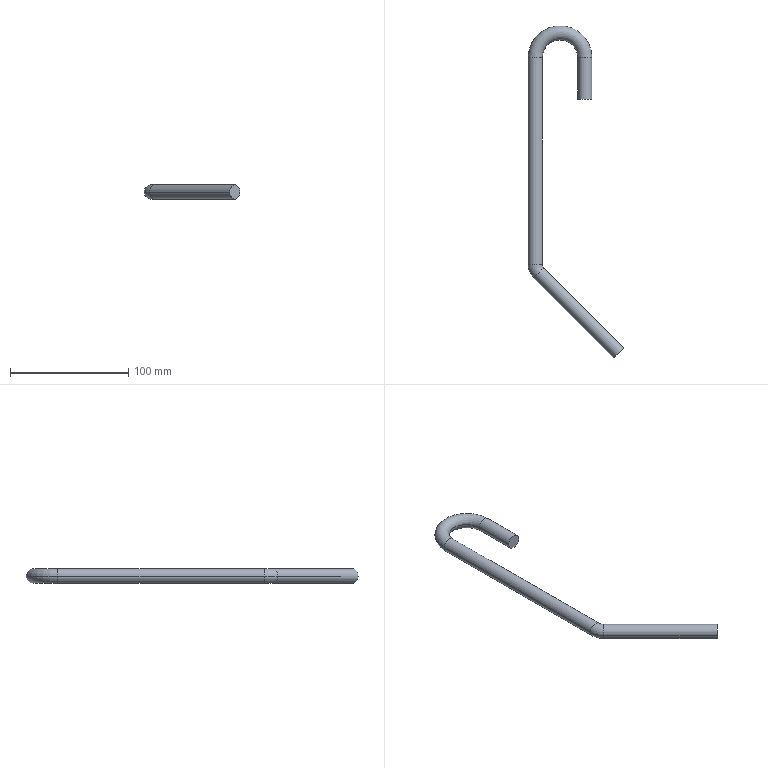Part | SolidWorks | features Sweep 1 | 1 solid | 12 faces | box 80.953 x 280.953 x 12 mm | volume 42925 mm3 | cylinder 6 | torus 4 | plane 2 | commonest cylinder face diameters 12 x6
STEP:
#1=CARTESIAN_POINT('',(-76.711,249.711,0.));
#2=VERTEX_POINT('',#1);
#3=CARTESIAN_POINT('',(-64.711,249.711,0.));
#4=VERTEX_POINT('',#3);
#5=CARTESIAN_POINT('',(-70.711,249.711,0.));
#6=DIRECTION('',(0.,-1.,0.));
#7=DIRECTION('',(0.,0.,1.));
#8=AXIS2_PLACEMENT_3D('',#5,#6,#7);
#9=CIRCLE('',#8,6.);
#10=EDGE_CURVE('',#2,#4,#9,.T.);
#11=ORIENTED_EDGE('',*,*,#10,.F.);
#12=CARTESIAN_POINT('',(-22.711,249.711,0.));
#13=VERTEX_POINT('',#12);
#14=CARTESIAN_POINT('',(-49.711,249.711,0.));
#15=DIRECTION('',(0.,0.,-1.));
#16=DIRECTION('',(-1.,0.,0.));
#17=AXIS2_PLACEMENT_3D('',#14,#15,#16);
#18=CIRCLE('',#17,27.);
#19=EDGE_CURVE('',#2,#13,#18,.T.);
#20=ORIENTED_EDGE('',*,*,#19,.T.);
#21=CARTESIAN_POINT('',(-34.711,249.711,0.));
#22=VERTEX_POINT('',#21);
#23=CARTESIAN_POINT('',(-28.711,249.711,0.));
#24=DIRECTION('',(0.,1.,0.));
#25=DIRECTION('',(0.,0.,1.));
#26=AXIS2_PLACEMENT_3D('',#23,#24,#25);
#27=CIRCLE('',#26,6.);
#28=EDGE_CURVE('',#13,#22,#27,.T.);
#29=ORIENTED_EDGE('',*,*,#28,.T.);
#30=CARTESIAN_POINT('',(-49.711,249.711,0.));
#31=DIRECTION('',(0.,0.,-1.));
#32=DIRECTION('',(-1.,0.,0.));
#33=AXIS2_PLACEMENT_3D('',#30,#31,#32);
#34=CIRCLE('',#33,15.);
#35=EDGE_CURVE('',#4,#22,#34,.T.);
#36=ORIENTED_EDGE('',*,*,#35,.F.);
#37=EDGE_LOOP('',(#11,#20,#29,#36));
#38=FACE_OUTER_BOUND('',#37,.T.);
#39=CARTESIAN_POINT('',(-49.711,249.711,0.));
#40=DIRECTION('',(0.,0.,-1.));
#41=DIRECTION('',(-1.,0.,0.));
#42=AXIS2_PLACEMENT_3D('',#39,#40,#41);
#43=TOROIDAL_SURFACE('',#42,21.,6.);
#44=ADVANCED_FACE('',(#38),#43,.T.);
#45=CARTESIAN_POINT('',(-72.024,63.539,0.));
#46=VERTEX_POINT('',#45);
#47=CARTESIAN_POINT('',(-63.539,72.024,0.));
#48=VERTEX_POINT('',#47);
#49=CARTESIAN_POINT('',(-67.782,67.782,0.));
#50=DIRECTION('',(0.7071,-0.7071,0.));
#51=DIRECTION('',(0.,0.,1.));
#52=AXIS2_PLACEMENT_3D('',#49,#50,#51);
#53=CIRCLE('',#52,6.);
#54=EDGE_CURVE('',#46,#48,#53,.T.);
#55=ORIENTED_EDGE('',*,*,#54,.F.);
#56=CARTESIAN_POINT('',(-76.711,74.853,0.));
#57=VERTEX_POINT('',#56);
#58=CARTESIAN_POINT('',(-60.711,74.853,0.));
#59=DIRECTION('',(0.,0.,-1.));
#60=DIRECTION('',(-1.,0.,0.));
#61=AXIS2_PLACEMENT_3D('',#58,#59,#60);
#62=CIRCLE('',#61,16.);
#63=EDGE_CURVE('',#46,#57,#62,.T.);
#64=ORIENTED_EDGE('',*,*,#63,.T.);
#65=CARTESIAN_POINT('',(-64.711,74.853,0.));
#66=VERTEX_POINT('',#65);
#67=CARTESIAN_POINT('',(-70.711,74.853,0.));
#68=DIRECTION('',(0.,-1.,0.));
#69=DIRECTION('',(0.,0.,1.));
#70=AXIS2_PLACEMENT_3D('',#67,#68,#69);
#71=CIRCLE('',#70,6.);
#72=EDGE_CURVE('',#57,#66,#71,.T.);
#73=ORIENTED_EDGE('',*,*,#72,.T.);
#74=CARTESIAN_POINT('',(-60.711,74.853,0.));
#75=DIRECTION('',(0.,0.,-1.));
#76=DIRECTION('',(-1.,0.,0.));
#77=AXIS2_PLACEMENT_3D('',#74,#75,#76);
#78=CIRCLE('',#77,4.);
#79=EDGE_CURVE('',#48,#66,#78,.T.);
#80=ORIENTED_EDGE('',*,*,#79,.F.);
#81=EDGE_LOOP('',(#55,#64,#73,#80));
#82=FACE_OUTER_BOUND('',#81,.T.);
#83=CARTESIAN_POINT('',(-60.711,74.853,0.));
#84=DIRECTION('',(0.,0.,-1.));
#85=DIRECTION('',(-1.,0.,0.));
#86=AXIS2_PLACEMENT_3D('',#83,#84,#85);
#87=TOROIDAL_SURFACE('',#86,10.,6.);
#88=ADVANCED_FACE('',(#82),#87,.T.);
#89=CARTESIAN_POINT('',(-28.711,249.711,0.));
#90=DIRECTION('',(0.,1.,0.));
#91=DIRECTION('',(0.,0.,1.));
#92=AXIS2_PLACEMENT_3D('',#89,#90,#91);
#93=CIRCLE('',#92,6.);
#94=EDGE_CURVE('',#22,#13,#93,.T.);
#95=ORIENTED_EDGE('',*,*,#94,.F.);
#96=CARTESIAN_POINT('',(-34.711,214.711,0.));
#97=VERTEX_POINT('',#96);
#98=CARTESIAN_POINT('',(-34.711,249.711,0.));
#99=DIRECTION('',(0.,-1.,0.));
#100=VECTOR('',#99,1000.);
#101=LINE('',#98,#100);
#102=EDGE_CURVE('',#22,#97,#101,.T.);
#103=ORIENTED_EDGE('',*,*,#102,.T.);
#104=CARTESIAN_POINT('',(-22.711,214.711,0.));
#105=VERTEX_POINT('',#104);
#106=CARTESIAN_POINT('',(-28.711,214.711,0.));
#107=DIRECTION('',(0.,1.,0.));
#108=DIRECTION('',(0.,0.,1.));
#109=AXIS2_PLACEMENT_3D('',#106,#107,#108);
#110=CIRCLE('',#109,6.);
#111=EDGE_CURVE('',#97,#105,#110,.T.);
#112=ORIENTED_EDGE('',*,*,#111,.T.);
#113=CARTESIAN_POINT('',(-22.711,249.711,0.));
#114=DIRECTION('',(0.,-1.,0.));
#115=VECTOR('',#114,1000.);
#116=LINE('',#113,#115);
#117=EDGE_CURVE('',#13,#105,#116,.T.);
#118=ORIENTED_EDGE('',*,*,#117,.F.);
#119=EDGE_LOOP('',(#95,#103,#112,#118));
#120=FACE_OUTER_BOUND('',#119,.T.);
#121=CARTESIAN_POINT('',(-28.711,249.711,0.));
#122=DIRECTION('',(0.,-1.,0.));
#123=DIRECTION('',(1.,0.,0.));
#124=AXIS2_PLACEMENT_3D('',#121,#122,#123);
#125=CYLINDRICAL_SURFACE('',#124,6.);
#126=ADVANCED_FACE('',(#120),#125,.T.);
#127=CARTESIAN_POINT('',(-70.711,74.853,0.));
#128=DIRECTION('',(0.,-1.,0.));
#129=DIRECTION('',(0.,0.,1.));
#130=AXIS2_PLACEMENT_3D('',#127,#128,#129);
#131=CIRCLE('',#130,6.);
#132=EDGE_CURVE('',#66,#57,#131,.T.);
#133=ORIENTED_EDGE('',*,*,#132,.F.);
#134=CARTESIAN_POINT('',(-64.711,74.853,0.));
#135=DIRECTION('',(0.,1.,0.));
#136=VECTOR('',#135,1000.);
#137=LINE('',#134,#136);
#138=EDGE_CURVE('',#66,#4,#137,.T.);
#139=ORIENTED_EDGE('',*,*,#138,.T.);
#140=CARTESIAN_POINT('',(-70.711,249.711,0.));
#141=DIRECTION('',(0.,-1.,0.));
#142=DIRECTION('',(0.,0.,1.));
#143=AXIS2_PLACEMENT_3D('',#140,#141,#142);
#144=CIRCLE('',#143,6.);
#145=EDGE_CURVE('',#4,#2,#144,.T.);
#146=ORIENTED_EDGE('',*,*,#145,.T.);
#147=CARTESIAN_POINT('',(-76.711,74.853,0.));
#148=DIRECTION('',(0.,1.,0.));
#149=VECTOR('',#148,1000.);
#150=LINE('',#147,#149);
#151=EDGE_CURVE('',#57,#2,#150,.T.);
#152=ORIENTED_EDGE('',*,*,#151,.F.);
#153=EDGE_LOOP('',(#133,#139,#146,#152));
#154=FACE_OUTER_BOUND('',#153,.T.);
#155=CARTESIAN_POINT('',(-70.711,74.853,0.));
#156=DIRECTION('',(0.,1.,0.));
#157=DIRECTION('',(-1.,0.,0.));
#158=AXIS2_PLACEMENT_3D('',#155,#156,#157);
#159=CYLINDRICAL_SURFACE('',#158,6.);
#160=ADVANCED_FACE('',(#154),#159,.T.);
#161=CARTESIAN_POINT('',(4.243,4.243,0.));
#162=VERTEX_POINT('',#161);
#163=CARTESIAN_POINT('',(-4.243,-4.243,0.));
#164=VERTEX_POINT('',#163);
#165=CARTESIAN_POINT('',(0.,0.,0.));
#166=DIRECTION('',(0.7071,-0.7071,0.));
#167=DIRECTION('',(0.,0.,1.));
#168=AXIS2_PLACEMENT_3D('',#165,#166,#167);
#169=CIRCLE('',#168,6.);
#170=EDGE_CURVE('',#162,#164,#169,.T.);
#171=ORIENTED_EDGE('',*,*,#170,.F.);
#172=CARTESIAN_POINT('',(4.243,4.243,0.));
#173=DIRECTION('',(-0.7071,0.7071,0.));
#174=VECTOR('',#173,1000.);
#175=LINE('',#172,#174);
#176=EDGE_CURVE('',#162,#48,#175,.T.);
#177=ORIENTED_EDGE('',*,*,#176,.T.);
#178=CARTESIAN_POINT('',(-67.782,67.782,0.));
#179=DIRECTION('',(0.7071,-0.7071,0.));
#180=DIRECTION('',(0.,0.,1.));
#181=AXIS2_PLACEMENT_3D('',#178,#179,#180);
#182=CIRCLE('',#181,6.);
#183=EDGE_CURVE('',#48,#46,#182,.T.);
#184=ORIENTED_EDGE('',*,*,#183,.T.);
#185=CARTESIAN_POINT('',(-4.243,-4.243,0.));
#186=DIRECTION('',(-0.7071,0.7071,0.));
#187=VECTOR('',#186,1000.);
#188=LINE('',#185,#187);
#189=EDGE_CURVE('',#164,#46,#188,.T.);
#190=ORIENTED_EDGE('',*,*,#189,.F.);
#191=EDGE_LOOP('',(#171,#177,#184,#190));
#192=FACE_OUTER_BOUND('',#191,.T.);
#193=CARTESIAN_POINT('',(0.,0.,0.));
#194=DIRECTION('',(-0.7071,0.7071,0.));
#195=DIRECTION('',(-0.7071,-0.7071,0.));
#196=AXIS2_PLACEMENT_3D('',#193,#194,#195);
#197=CYLINDRICAL_SURFACE('',#196,6.);
#198=ADVANCED_FACE('',(#192),#197,.T.);
#199=ORIENTED_EDGE('',*,*,#102,.F.);
#200=ORIENTED_EDGE('',*,*,#28,.F.);
#201=ORIENTED_EDGE('',*,*,#117,.T.);
#202=CARTESIAN_POINT('',(-28.711,214.711,0.));
#203=DIRECTION('',(0.,1.,0.));
#204=DIRECTION('',(0.,0.,1.));
#205=AXIS2_PLACEMENT_3D('',#202,#203,#204);
#206=CIRCLE('',#205,6.);
#207=EDGE_CURVE('',#105,#97,#206,.T.);
#208=ORIENTED_EDGE('',*,*,#207,.T.);
#209=EDGE_LOOP('',(#199,#200,#201,#208));
#210=FACE_OUTER_BOUND('',#209,.T.);
#211=CARTESIAN_POINT('',(-28.711,249.711,0.));
#212=DIRECTION('',(0.,-1.,0.));
#213=DIRECTION('',(1.,0.,0.));
#214=AXIS2_PLACEMENT_3D('',#211,#212,#213);
#215=CYLINDRICAL_SURFACE('',#214,6.);
#216=ADVANCED_FACE('',(#210),#215,.T.);
#217=ORIENTED_EDGE('',*,*,#19,.F.);
#218=ORIENTED_EDGE('',*,*,#145,.F.);
#219=ORIENTED_EDGE('',*,*,#35,.T.);
#220=ORIENTED_EDGE('',*,*,#94,.T.);
#221=EDGE_LOOP('',(#217,#218,#219,#220));
#222=FACE_OUTER_BOUND('',#221,.T.);
#223=CARTESIAN_POINT('',(-49.711,249.711,0.));
#224=DIRECTION('',(0.,0.,-1.));
#225=DIRECTION('',(-1.,0.,0.));
#226=AXIS2_PLACEMENT_3D('',#223,#224,#225);
#227=TOROIDAL_SURFACE('',#226,21.,6.);
#228=ADVANCED_FACE('',(#222),#227,.T.);
#229=ORIENTED_EDGE('',*,*,#138,.F.);
#230=ORIENTED_EDGE('',*,*,#72,.F.);
#231=ORIENTED_EDGE('',*,*,#151,.T.);
#232=ORIENTED_EDGE('',*,*,#10,.T.);
#233=EDGE_LOOP('',(#229,#230,#231,#232));
#234=FACE_OUTER_BOUND('',#233,.T.);
#235=CARTESIAN_POINT('',(-70.711,74.853,0.));
#236=DIRECTION('',(0.,1.,0.));
#237=DIRECTION('',(-1.,0.,0.));
#238=AXIS2_PLACEMENT_3D('',#235,#236,#237);
#239=CYLINDRICAL_SURFACE('',#238,6.);
#240=ADVANCED_FACE('',(#234),#239,.T.);
#241=ORIENTED_EDGE('',*,*,#63,.F.);
#242=ORIENTED_EDGE('',*,*,#183,.F.);
#243=ORIENTED_EDGE('',*,*,#79,.T.);
#244=ORIENTED_EDGE('',*,*,#132,.T.);
#245=EDGE_LOOP('',(#241,#242,#243,#244));
#246=FACE_OUTER_BOUND('',#245,.T.);
#247=CARTESIAN_POINT('',(-60.711,74.853,0.));
#248=DIRECTION('',(0.,0.,-1.));
#249=DIRECTION('',(-1.,0.,0.));
#250=AXIS2_PLACEMENT_3D('',#247,#248,#249);
#251=TOROIDAL_SURFACE('',#250,10.,6.);
#252=ADVANCED_FACE('',(#246),#251,.T.);
#253=ORIENTED_EDGE('',*,*,#176,.F.);
#254=CARTESIAN_POINT('',(0.,0.,0.));
#255=DIRECTION('',(0.7071,-0.7071,0.));
#256=DIRECTION('',(0.,0.,1.));
#257=AXIS2_PLACEMENT_3D('',#254,#255,#256);
#258=CIRCLE('',#257,6.);
#259=EDGE_CURVE('',#164,#162,#258,.T.);
#260=ORIENTED_EDGE('',*,*,#259,.F.);
#261=ORIENTED_EDGE('',*,*,#189,.T.);
#262=ORIENTED_EDGE('',*,*,#54,.T.);
#263=EDGE_LOOP('',(#253,#260,#261,#262));
#264=FACE_OUTER_BOUND('',#263,.T.);
#265=CARTESIAN_POINT('',(0.,0.,0.));
#266=DIRECTION('',(-0.7071,0.7071,0.));
#267=DIRECTION('',(-0.7071,-0.7071,0.));
#268=AXIS2_PLACEMENT_3D('',#265,#266,#267);
#269=CYLINDRICAL_SURFACE('',#268,6.);
#270=ADVANCED_FACE('',(#264),#269,.T.);
#271=ORIENTED_EDGE('',*,*,#207,.F.);
#272=ORIENTED_EDGE('',*,*,#111,.F.);
#273=EDGE_LOOP('',(#271,#272));
#274=FACE_OUTER_BOUND('',#273,.T.);
#275=CARTESIAN_POINT('',(-28.711,214.711,0.));
#276=DIRECTION('',(0.,1.,0.));
#277=DIRECTION('',(0.,0.,1.));
#278=AXIS2_PLACEMENT_3D('',#275,#276,#277);
#279=PLANE('',#278);
#280=ADVANCED_FACE('',(#274),#279,.F.);
#281=ORIENTED_EDGE('',*,*,#259,.T.);
#282=ORIENTED_EDGE('',*,*,#170,.T.);
#283=EDGE_LOOP('',(#281,#282));
#284=FACE_OUTER_BOUND('',#283,.T.);
#285=CARTESIAN_POINT('',(0.,0.,0.));
#286=DIRECTION('',(0.7071,-0.7071,0.));
#287=DIRECTION('',(0.,0.,1.));
#288=AXIS2_PLACEMENT_3D('',#285,#286,#287);
#289=PLANE('',#288);
#290=ADVANCED_FACE('',(#284),#289,.T.);
#291=CLOSED_SHELL('',(#44,#88,#126,#160,#198,#216,#228,#240,#252,#270,#280,#290));
#292=MANIFOLD_SOLID_BREP('',#291);
#293=CARTESIAN_POINT('',(0.,0.,0.));
#294=DIRECTION('',(0.,0.,1.));
#295=DIRECTION('',(1.,0.,0.));
#296=AXIS2_PLACEMENT_3D('',#293,#294,#295);
#297=(LENGTH_UNIT()NAMED_UNIT(*)SI_UNIT(.MILLI.,.METRE.));
#298=UNCERTAINTY_MEASURE_WITH_UNIT(LENGTH_MEASURE(0.00001),#297,'','');
#299=(NAMED_UNIT(*)PLANE_ANGLE_UNIT()SI_UNIT($,.RADIAN.));
#300=(NAMED_UNIT(*)SI_UNIT($,.STERADIAN.)SOLID_ANGLE_UNIT());
#301=(GEOMETRIC_REPRESENTATION_CONTEXT(3)GLOBAL_UNCERTAINTY_ASSIGNED_CONTEXT((#298))GLOBAL_UNIT_ASSIGNED_CONTEXT((#297,#299,#300))REPRESENTATION_CONTEXT('',''));
#302=ADVANCED_BREP_SHAPE_REPRESENTATION('',(#292,#296),#301);